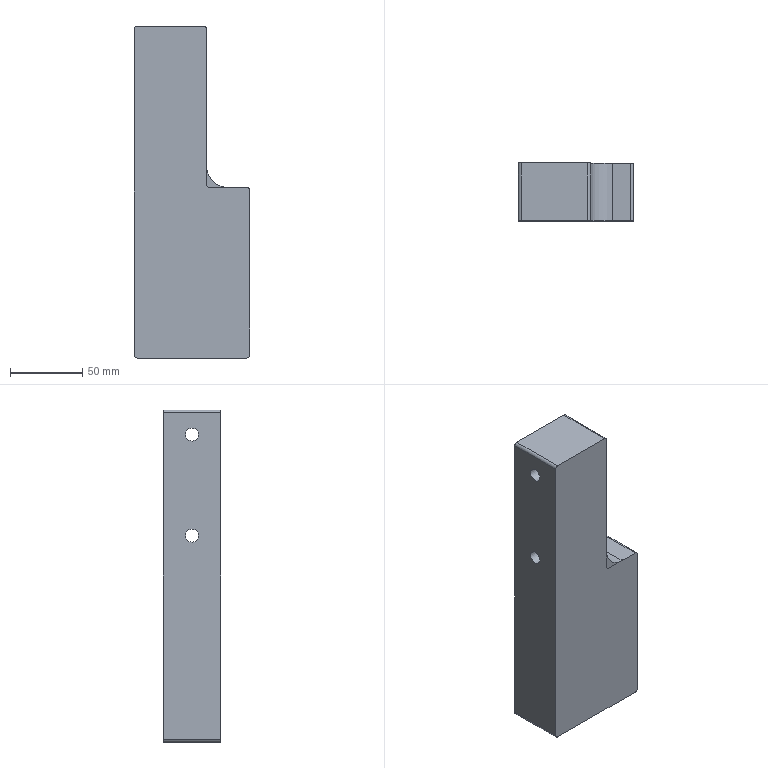Part | 2 solids | 64 faces | box 80 x 40 x 230 mm | volume 1173867 mm3 | cylinder 30 | plane 22 | cone 12 | commonest cylinder face diameters 4 x11 6.8 x8 9 x4 15 x4 15.5 x2 30 x1